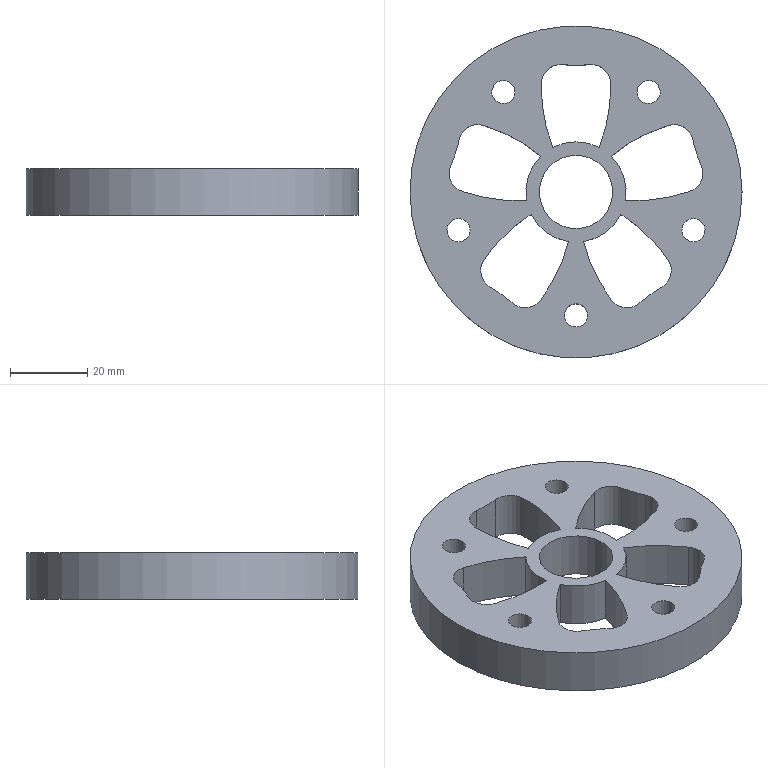Part | NX | features DATUM_CSYS 4, EXTRUDE 4, SKETCH 3 | 1 solid | 39 faces | box 86 x 86 x 12 mm | volume 44699 mm3 | cylinder 37 | plane 2 | commonest cylinder face diameters 86 x11 10 x10 6 x5 26 x5 70 x5 19 x1
STEP:
#1=CARTESIAN_POINT('',(43.,0.,-12.));
#2=VERTEX_POINT('',#1);
#3=CARTESIAN_POINT('',(0.,0.,-12.));
#4=DIRECTION('',(0.,0.,1.));
#5=DIRECTION('',(1.,0.,0.));
#6=AXIS2_PLACEMENT_3D('',#3,#4,#5);
#7=CIRCLE('',#6,43.);
#8=EDGE_CURVE('',#2,#2,#7,.T.);
#9=ORIENTED_EDGE('',*,*,#8,.T.);
#10=EDGE_LOOP('',(#9));
#11=FACE_BOUND('',#10,.T.);
#12=CARTESIAN_POINT('',(43.,0.,0.));
#13=VERTEX_POINT('',#12);
#14=CARTESIAN_POINT('',(0.,0.,0.));
#15=DIRECTION('',(0.,0.,1.));
#16=DIRECTION('',(1.,0.,0.));
#17=AXIS2_PLACEMENT_3D('',#14,#15,#16);
#18=CIRCLE('',#17,43.);
#19=EDGE_CURVE('',#13,#13,#18,.T.);
#20=ORIENTED_EDGE('',*,*,#19,.F.);
#21=EDGE_LOOP('',(#20));
#22=FACE_BOUND('',#21,.T.);
#23=CARTESIAN_POINT('',(0.,0.,-12.));
#24=DIRECTION('',(0.,0.,1.));
#25=DIRECTION('',(1.,0.,0.));
#26=AXIS2_PLACEMENT_3D('',#23,#24,#25);
#27=CYLINDRICAL_SURFACE('',#26,43.);
#28=ADVANCED_FACE('',(#11,#22),#27,.T.);
#29=CARTESIAN_POINT('',(9.5,0.,-12.));
#30=VERTEX_POINT('',#29);
#31=CARTESIAN_POINT('',(0.,0.,-12.));
#32=DIRECTION('',(0.,0.,1.));
#33=DIRECTION('',(1.,0.,0.));
#34=AXIS2_PLACEMENT_3D('',#31,#32,#33);
#35=CIRCLE('',#34,9.5);
#36=EDGE_CURVE('',#30,#30,#35,.T.);
#37=ORIENTED_EDGE('',*,*,#36,.F.);
#38=EDGE_LOOP('',(#37));
#39=FACE_BOUND('',#38,.T.);
#40=CARTESIAN_POINT('',(9.5,0.,0.));
#41=VERTEX_POINT('',#40);
#42=CARTESIAN_POINT('',(0.,0.,0.));
#43=DIRECTION('',(0.,0.,1.));
#44=DIRECTION('',(1.,0.,0.));
#45=AXIS2_PLACEMENT_3D('',#42,#43,#44);
#46=CIRCLE('',#45,9.5);
#47=EDGE_CURVE('',#41,#41,#46,.T.);
#48=ORIENTED_EDGE('',*,*,#47,.T.);
#49=EDGE_LOOP('',(#48));
#50=FACE_BOUND('',#49,.T.);
#51=CARTESIAN_POINT('',(0.,0.,-12.));
#52=DIRECTION('',(0.,0.,1.));
#53=DIRECTION('',(1.,0.,0.));
#54=AXIS2_PLACEMENT_3D('',#51,#52,#53);
#55=CYLINDRICAL_SURFACE('',#54,9.5);
#56=ADVANCED_FACE('',(#39,#50),#55,.F.);
#57=CARTESIAN_POINT('',(31.361,-7.035,-12.));
#58=VERTEX_POINT('',#57);
#59=CARTESIAN_POINT('',(30.434,-9.889,-12.));
#60=DIRECTION('',(0.,0.,1.));
#61=DIRECTION('',(0.309,0.9511,0.));
#62=AXIS2_PLACEMENT_3D('',#59,#60,#61);
#63=CIRCLE('',#62,3.);
#64=EDGE_CURVE('',#58,#58,#63,.T.);
#65=ORIENTED_EDGE('',*,*,#64,.T.);
#66=EDGE_LOOP('',(#65));
#67=FACE_BOUND('',#66,.T.);
#68=CARTESIAN_POINT('',(16.382,27.652,-12.));
#69=VERTEX_POINT('',#68);
#70=CARTESIAN_POINT('',(18.809,25.889,-12.));
#71=DIRECTION('',(0.,0.,1.));
#72=DIRECTION('',(-0.809,0.5878,0.));
#73=AXIS2_PLACEMENT_3D('',#70,#71,#72);
#74=CIRCLE('',#73,3.);
#75=EDGE_CURVE('',#69,#69,#74,.T.);
#76=ORIENTED_EDGE('',*,*,#75,.T.);
#77=EDGE_LOOP('',(#76));
#78=FACE_BOUND('',#77,.T.);
#79=CARTESIAN_POINT('',(3.,-32.,-12.));
#80=VERTEX_POINT('',#79);
#81=CARTESIAN_POINT('',(0.,-32.,-12.));
#82=DIRECTION('',(0.,0.,1.));
#83=DIRECTION('',(1.,0.,0.));
#84=AXIS2_PLACEMENT_3D('',#81,#82,#83);
#85=CIRCLE('',#84,3.);
#86=EDGE_CURVE('',#80,#80,#85,.T.);
#87=ORIENTED_EDGE('',*,*,#86,.T.);
#88=EDGE_LOOP('',(#87));
#89=FACE_BOUND('',#88,.T.);
#90=CARTESIAN_POINT('',(-21.236,24.125,-12.));
#91=VERTEX_POINT('',#90);
#92=CARTESIAN_POINT('',(-18.809,25.889,-12.));
#93=DIRECTION('',(0.,0.,1.));
#94=DIRECTION('',(-0.809,-0.5878,0.));
#95=AXIS2_PLACEMENT_3D('',#92,#93,#94);
#96=CIRCLE('',#95,3.);
#97=EDGE_CURVE('',#91,#91,#96,.T.);
#98=ORIENTED_EDGE('',*,*,#97,.T.);
#99=EDGE_LOOP('',(#98));
#100=FACE_BOUND('',#99,.T.);
#101=CARTESIAN_POINT('',(-29.507,-12.742,-12.));
#102=VERTEX_POINT('',#101);
#103=CARTESIAN_POINT('',(-30.434,-9.889,-12.));
#104=DIRECTION('',(0.,0.,1.));
#105=DIRECTION('',(0.309,-0.9511,0.));
#106=AXIS2_PLACEMENT_3D('',#103,#104,#105);
#107=CIRCLE('',#106,3.);
#108=EDGE_CURVE('',#102,#102,#107,.T.);
#109=ORIENTED_EDGE('',*,*,#108,.T.);
#110=EDGE_LOOP('',(#109));
#111=FACE_BOUND('',#110,.T.);
#112=CARTESIAN_POINT('',(-23.933,17.239,-12.));
#113=VERTEX_POINT('',#112);
#114=CARTESIAN_POINT('',(-30.279,13.519,-12.));
#115=VERTEX_POINT('',#114);
#116=CARTESIAN_POINT('',(-25.394,12.457,-12.));
#117=DIRECTION('',(0.,0.,1.));
#118=DIRECTION('',(1.,0.,0.));
#119=AXIS2_PLACEMENT_3D('',#116,#117,#118);
#120=CIRCLE('',#119,5.);
#121=EDGE_CURVE('',#113,#115,#120,.T.);
#122=ORIENTED_EDGE('',*,*,#121,.T.);
#123=CARTESIAN_POINT('',(-32.443,6.861,-12.));
#124=VERTEX_POINT('',#123);
#125=CARTESIAN_POINT('',(-64.481,20.951,-12.));
#126=DIRECTION('',(0.,0.,1.));
#127=DIRECTION('',(1.,0.,0.));
#128=AXIS2_PLACEMENT_3D('',#125,#126,#127);
#129=CIRCLE('',#128,35.);
#130=EDGE_CURVE('',#115,#124,#129,.F.);
#131=ORIENTED_EDGE('',*,*,#130,.T.);
#132=CARTESIAN_POINT('',(-29.495,0.1211,-12.));
#133=VERTEX_POINT('',#132);
#134=CARTESIAN_POINT('',(-27.866,4.848,-12.));
#135=DIRECTION('',(0.,0.,1.));
#136=DIRECTION('',(1.,0.,0.));
#137=AXIS2_PLACEMENT_3D('',#134,#135,#136);
#138=CIRCLE('',#137,5.);
#139=EDGE_CURVE('',#124,#133,#138,.T.);
#140=ORIENTED_EDGE('',*,*,#139,.T.);
#141=CARTESIAN_POINT('',(-12.822,-2.143,-12.));
#142=VERTEX_POINT('',#141);
#143=CARTESIAN_POINT('',(-15.485,40.775,-12.));
#144=DIRECTION('',(0.,0.,1.));
#145=DIRECTION('',(1.,0.,0.));
#146=AXIS2_PLACEMENT_3D('',#143,#144,#145);
#147=CIRCLE('',#146,43.);
#148=EDGE_CURVE('',#133,#142,#147,.T.);
#149=ORIENTED_EDGE('',*,*,#148,.T.);
#150=CARTESIAN_POINT('',(-9.114,9.27,-12.));
#151=VERTEX_POINT('',#150);
#152=CARTESIAN_POINT('',(0.,0.,-12.));
#153=DIRECTION('',(0.,0.,1.));
#154=DIRECTION('',(1.,0.,0.));
#155=AXIS2_PLACEMENT_3D('',#152,#153,#154);
#156=CIRCLE('',#155,13.);
#157=EDGE_CURVE('',#142,#151,#156,.F.);
#158=ORIENTED_EDGE('',*,*,#157,.T.);
#159=CARTESIAN_POINT('',(-36.495,-23.886,-12.));
#160=DIRECTION('',(0.,0.,1.));
#161=DIRECTION('',(1.,0.,0.));
#162=AXIS2_PLACEMENT_3D('',#159,#160,#161);
#163=CIRCLE('',#162,43.);
#164=EDGE_CURVE('',#151,#113,#163,.T.);
#165=ORIENTED_EDGE('',*,*,#164,.T.);
#166=EDGE_LOOP('',(#122,#131,#140,#149,#158,#165));
#167=FACE_BOUND('',#166,.T.);
#168=CARTESIAN_POINT('',(-11.633,-5.803,-12.));
#169=VERTEX_POINT('',#168);
#170=CARTESIAN_POINT('',(-23.791,-17.434,-12.));
#171=VERTEX_POINT('',#170);
#172=CARTESIAN_POINT('',(11.439,-42.09,-12.));
#173=DIRECTION('',(0.,0.,1.));
#174=DIRECTION('',(1.,0.,0.));
#175=AXIS2_PLACEMENT_3D('',#172,#173,#174);
#176=CIRCLE('',#175,43.);
#177=EDGE_CURVE('',#169,#171,#176,.T.);
#178=ORIENTED_EDGE('',*,*,#177,.T.);
#179=CARTESIAN_POINT('',(-22.214,-24.62,-12.));
#180=VERTEX_POINT('',#179);
#181=CARTESIAN_POINT('',(-19.694,-20.301,-12.));
#182=DIRECTION('',(0.,0.,1.));
#183=DIRECTION('',(1.,0.,0.));
#184=AXIS2_PLACEMENT_3D('',#181,#182,#183);
#185=CIRCLE('',#184,5.);
#186=EDGE_CURVE('',#171,#180,#185,.T.);
#187=ORIENTED_EDGE('',*,*,#186,.T.);
#188=CARTESIAN_POINT('',(-16.551,-28.735,-12.));
#189=VERTEX_POINT('',#188);
#190=CARTESIAN_POINT('',(-39.852,-54.851,-12.));
#191=DIRECTION('',(0.,0.,1.));
#192=DIRECTION('',(1.,0.,0.));
#193=AXIS2_PLACEMENT_3D('',#190,#191,#192);
#194=CIRCLE('',#193,35.);
#195=EDGE_CURVE('',#180,#189,#194,.F.);
#196=ORIENTED_EDGE('',*,*,#195,.T.);
#197=CARTESIAN_POINT('',(-9.229,-28.014,-12.));
#198=VERTEX_POINT('',#197);
#199=CARTESIAN_POINT('',(-13.222,-25.004,-12.));
#200=DIRECTION('',(0.,0.,1.));
#201=DIRECTION('',(1.,0.,0.));
#202=AXIS2_PLACEMENT_3D('',#199,#200,#201);
#203=CIRCLE('',#202,5.);
#204=EDGE_CURVE('',#189,#198,#203,.T.);
#205=ORIENTED_EDGE('',*,*,#204,.T.);
#206=CARTESIAN_POINT('',(-1.925,-12.857,-12.));
#207=VERTEX_POINT('',#206);
#208=CARTESIAN_POINT('',(-43.564,-2.127,-12.));
#209=DIRECTION('',(0.,0.,1.));
#210=DIRECTION('',(1.,0.,0.));
#211=AXIS2_PLACEMENT_3D('',#208,#209,#210);
#212=CIRCLE('',#211,43.);
#213=EDGE_CURVE('',#198,#207,#212,.T.);
#214=ORIENTED_EDGE('',*,*,#213,.T.);
#215=CARTESIAN_POINT('',(0.,0.,-12.));
#216=DIRECTION('',(0.,0.,1.));
#217=DIRECTION('',(1.,0.,0.));
#218=AXIS2_PLACEMENT_3D('',#215,#216,#217);
#219=CIRCLE('',#218,13.);
#220=EDGE_CURVE('',#207,#169,#219,.F.);
#221=ORIENTED_EDGE('',*,*,#220,.T.);
#222=EDGE_LOOP('',(#178,#187,#196,#205,#214,#221));
#223=FACE_BOUND('',#222,.T.);
#224=CARTESIAN_POINT('',(-8.999,28.089,-12.));
#225=VERTEX_POINT('',#224);
#226=CARTESIAN_POINT('',(-6.,11.533,-12.));
#227=VERTEX_POINT('',#226);
#228=CARTESIAN_POINT('',(33.994,27.327,-12.));
#229=DIRECTION('',(0.,0.,1.));
#230=DIRECTION('',(1.,0.,0.));
#231=AXIS2_PLACEMENT_3D('',#228,#229,#230);
#232=CIRCLE('',#231,43.);
#233=EDGE_CURVE('',#225,#227,#232,.T.);
#234=ORIENTED_EDGE('',*,*,#233,.T.);
#235=CARTESIAN_POINT('',(6.,11.533,-12.));
#236=VERTEX_POINT('',#235);
#237=CARTESIAN_POINT('',(0.,0.,-12.));
#238=DIRECTION('',(0.,0.,1.));
#239=DIRECTION('',(1.,0.,0.));
#240=AXIS2_PLACEMENT_3D('',#237,#238,#239);
#241=CIRCLE('',#240,13.);
#242=EDGE_CURVE('',#227,#236,#241,.F.);
#243=ORIENTED_EDGE('',*,*,#242,.T.);
#244=CARTESIAN_POINT('',(8.999,28.089,-12.));
#245=VERTEX_POINT('',#244);
#246=CARTESIAN_POINT('',(-33.994,27.327,-12.));
#247=DIRECTION('',(0.,0.,1.));
#248=DIRECTION('',(1.,0.,0.));
#249=AXIS2_PLACEMENT_3D('',#246,#247,#248);
#250=CIRCLE('',#249,43.);
#251=EDGE_CURVE('',#236,#245,#250,.T.);
#252=ORIENTED_EDGE('',*,*,#251,.T.);
#253=CARTESIAN_POINT('',(3.5,32.975,-12.));
#254=VERTEX_POINT('',#253);
#255=CARTESIAN_POINT('',(4.,28.,-12.));
#256=DIRECTION('',(0.,0.,1.));
#257=DIRECTION('',(1.,0.,0.));
#258=AXIS2_PLACEMENT_3D('',#255,#256,#257);
#259=CIRCLE('',#258,5.);
#260=EDGE_CURVE('',#245,#254,#259,.T.);
#261=ORIENTED_EDGE('',*,*,#260,.T.);
#262=CARTESIAN_POINT('',(-3.5,32.975,-12.));
#263=VERTEX_POINT('',#262);
#264=CARTESIAN_POINT('',(0.,67.799,-12.));
#265=DIRECTION('',(0.,0.,1.));
#266=DIRECTION('',(1.,0.,0.));
#267=AXIS2_PLACEMENT_3D('',#264,#265,#266);
#268=CIRCLE('',#267,35.);
#269=EDGE_CURVE('',#254,#263,#268,.F.);
#270=ORIENTED_EDGE('',*,*,#269,.T.);
#271=CARTESIAN_POINT('',(-4.,28.,-12.));
#272=DIRECTION('',(0.,0.,1.));
#273=DIRECTION('',(1.,0.,0.));
#274=AXIS2_PLACEMENT_3D('',#271,#272,#273);
#275=CIRCLE('',#274,5.);
#276=EDGE_CURVE('',#263,#225,#275,.T.);
#277=ORIENTED_EDGE('',*,*,#276,.T.);
#278=EDGE_LOOP('',(#234,#243,#252,#261,#270,#277));
#279=FACE_BOUND('',#278,.T.);
#280=CARTESIAN_POINT('',(11.633,-5.803,-12.));
#281=VERTEX_POINT('',#280);
#282=CARTESIAN_POINT('',(1.925,-12.857,-12.));
#283=VERTEX_POINT('',#282);
#284=CARTESIAN_POINT('',(0.,0.,-12.));
#285=DIRECTION('',(0.,0.,1.));
#286=DIRECTION('',(1.,0.,0.));
#287=AXIS2_PLACEMENT_3D('',#284,#285,#286);
#288=CIRCLE('',#287,13.);
#289=EDGE_CURVE('',#281,#283,#288,.F.);
#290=ORIENTED_EDGE('',*,*,#289,.T.);
#291=CARTESIAN_POINT('',(9.229,-28.014,-12.));
#292=VERTEX_POINT('',#291);
#293=CARTESIAN_POINT('',(43.564,-2.127,-12.));
#294=DIRECTION('',(0.,0.,1.));
#295=DIRECTION('',(1.,0.,0.));
#296=AXIS2_PLACEMENT_3D('',#293,#294,#295);
#297=CIRCLE('',#296,43.);
#298=EDGE_CURVE('',#283,#292,#297,.T.);
#299=ORIENTED_EDGE('',*,*,#298,.T.);
#300=CARTESIAN_POINT('',(16.551,-28.735,-12.));
#301=VERTEX_POINT('',#300);
#302=CARTESIAN_POINT('',(13.222,-25.004,-12.));
#303=DIRECTION('',(0.,0.,1.));
#304=DIRECTION('',(1.,0.,0.));
#305=AXIS2_PLACEMENT_3D('',#302,#303,#304);
#306=CIRCLE('',#305,5.);
#307=EDGE_CURVE('',#292,#301,#306,.T.);
#308=ORIENTED_EDGE('',*,*,#307,.T.);
#309=CARTESIAN_POINT('',(22.214,-24.62,-12.));
#310=VERTEX_POINT('',#309);
#311=CARTESIAN_POINT('',(39.852,-54.851,-12.));
#312=DIRECTION('',(0.,0.,1.));
#313=DIRECTION('',(1.,0.,0.));
#314=AXIS2_PLACEMENT_3D('',#311,#312,#313);
#315=CIRCLE('',#314,35.);
#316=EDGE_CURVE('',#301,#310,#315,.F.);
#317=ORIENTED_EDGE('',*,*,#316,.T.);
#318=CARTESIAN_POINT('',(23.791,-17.434,-12.));
#319=VERTEX_POINT('',#318);
#320=CARTESIAN_POINT('',(19.694,-20.301,-12.));
#321=DIRECTION('',(0.,0.,1.));
#322=DIRECTION('',(1.,0.,0.));
#323=AXIS2_PLACEMENT_3D('',#320,#321,#322);
#324=CIRCLE('',#323,5.);
#325=EDGE_CURVE('',#310,#319,#324,.T.);
#326=ORIENTED_EDGE('',*,*,#325,.T.);
#327=CARTESIAN_POINT('',(-11.439,-42.09,-12.));
#328=DIRECTION('',(0.,0.,1.));
#329=DIRECTION('',(1.,0.,0.));
#330=AXIS2_PLACEMENT_3D('',#327,#328,#329);
#331=CIRCLE('',#330,43.);
#332=EDGE_CURVE('',#319,#281,#331,.T.);
#333=ORIENTED_EDGE('',*,*,#332,.T.);
#334=EDGE_LOOP('',(#290,#299,#308,#317,#326,#333));
#335=FACE_BOUND('',#334,.T.);
#336=CARTESIAN_POINT('',(23.933,17.239,-12.));
#337=VERTEX_POINT('',#336);
#338=CARTESIAN_POINT('',(9.114,9.27,-12.));
#339=VERTEX_POINT('',#338);
#340=CARTESIAN_POINT('',(36.495,-23.886,-12.));
#341=DIRECTION('',(0.,0.,1.));
#342=DIRECTION('',(1.,0.,0.));
#343=AXIS2_PLACEMENT_3D('',#340,#341,#342);
#344=CIRCLE('',#343,43.);
#345=EDGE_CURVE('',#337,#339,#344,.T.);
#346=ORIENTED_EDGE('',*,*,#345,.T.);
#347=CARTESIAN_POINT('',(12.822,-2.143,-12.));
#348=VERTEX_POINT('',#347);
#349=CARTESIAN_POINT('',(0.,0.,-12.));
#350=DIRECTION('',(0.,0.,1.));
#351=DIRECTION('',(1.,0.,0.));
#352=AXIS2_PLACEMENT_3D('',#349,#350,#351);
#353=CIRCLE('',#352,13.);
#354=EDGE_CURVE('',#339,#348,#353,.F.);
#355=ORIENTED_EDGE('',*,*,#354,.T.);
#356=CARTESIAN_POINT('',(29.495,0.1211,-12.));
#357=VERTEX_POINT('',#356);
#358=CARTESIAN_POINT('',(15.485,40.775,-12.));
#359=DIRECTION('',(0.,0.,1.));
#360=DIRECTION('',(1.,0.,0.));
#361=AXIS2_PLACEMENT_3D('',#358,#359,#360);
#362=CIRCLE('',#361,43.);
#363=EDGE_CURVE('',#348,#357,#362,.T.);
#364=ORIENTED_EDGE('',*,*,#363,.T.);
#365=CARTESIAN_POINT('',(32.443,6.861,-12.));
#366=VERTEX_POINT('',#365);
#367=CARTESIAN_POINT('',(27.866,4.848,-12.));
#368=DIRECTION('',(0.,0.,1.));
#369=DIRECTION('',(1.,0.,0.));
#370=AXIS2_PLACEMENT_3D('',#367,#368,#369);
#371=CIRCLE('',#370,5.);
#372=EDGE_CURVE('',#357,#366,#371,.T.);
#373=ORIENTED_EDGE('',*,*,#372,.T.);
#374=CARTESIAN_POINT('',(30.279,13.519,-12.));
#375=VERTEX_POINT('',#374);
#376=CARTESIAN_POINT('',(64.481,20.951,-12.));
#377=DIRECTION('',(0.,0.,1.));
#378=DIRECTION('',(1.,0.,0.));
#379=AXIS2_PLACEMENT_3D('',#376,#377,#378);
#380=CIRCLE('',#379,35.);
#381=EDGE_CURVE('',#366,#375,#380,.F.);
#382=ORIENTED_EDGE('',*,*,#381,.T.);
#383=CARTESIAN_POINT('',(25.394,12.457,-12.));
#384=DIRECTION('',(0.,0.,1.));
#385=DIRECTION('',(1.,0.,0.));
#386=AXIS2_PLACEMENT_3D('',#383,#384,#385);
#387=CIRCLE('',#386,5.);
#388=EDGE_CURVE('',#375,#337,#387,.T.);
#389=ORIENTED_EDGE('',*,*,#388,.T.);
#390=EDGE_LOOP('',(#346,#355,#364,#373,#382,#389));
#391=FACE_BOUND('',#390,.T.);
#392=ORIENTED_EDGE('',*,*,#8,.F.);
#393=EDGE_LOOP('',(#392));
#394=FACE_BOUND('',#393,.T.);
#395=ORIENTED_EDGE('',*,*,#36,.T.);
#396=EDGE_LOOP('',(#395));
#397=FACE_BOUND('',#396,.T.);
#398=CARTESIAN_POINT('',(0.,0.,-12.));
#399=DIRECTION('',(0.,0.,1.));
#400=DIRECTION('',(1.,0.,0.));
#401=AXIS2_PLACEMENT_3D('',#398,#399,#400);
#402=PLANE('',#401);
#403=ADVANCED_FACE('',(#67,#78,#89,#100,#111,#167,#223,#279,#335,#391,#394,#397),#402,.F.);
#404=CARTESIAN_POINT('',(9.114,9.27,0.));
#405=VERTEX_POINT('',#404);
#406=CARTESIAN_POINT('',(12.822,-2.143,0.));
#407=VERTEX_POINT('',#406);
#408=CARTESIAN_POINT('',(0.,0.,0.));
#409=DIRECTION('',(0.,0.,-1.));
#410=DIRECTION('',(0.309,-0.9511,0.));
#411=AXIS2_PLACEMENT_3D('',#408,#409,#410);
#412=CIRCLE('',#411,13.);
#413=EDGE_CURVE('',#405,#407,#412,.T.);
#414=ORIENTED_EDGE('',*,*,#413,.F.);
#415=CARTESIAN_POINT('',(23.933,17.239,0.));
#416=VERTEX_POINT('',#415);
#417=CARTESIAN_POINT('',(36.495,-23.886,0.));
#418=DIRECTION('',(0.,0.,1.));
#419=DIRECTION('',(0.309,-0.9511,0.));
#420=AXIS2_PLACEMENT_3D('',#417,#418,#419);
#421=CIRCLE('',#420,43.);
#422=EDGE_CURVE('',#416,#405,#421,.T.);
#423=ORIENTED_EDGE('',*,*,#422,.F.);
#424=CARTESIAN_POINT('',(30.279,13.519,0.));
#425=VERTEX_POINT('',#424);
#426=CARTESIAN_POINT('',(25.394,12.457,0.));
#427=DIRECTION('',(0.,0.,1.));
#428=DIRECTION('',(0.309,-0.9511,0.));
#429=AXIS2_PLACEMENT_3D('',#426,#427,#428);
#430=CIRCLE('',#429,5.);
#431=EDGE_CURVE('',#425,#416,#430,.T.);
#432=ORIENTED_EDGE('',*,*,#431,.F.);
#433=CARTESIAN_POINT('',(32.443,6.861,0.));
#434=VERTEX_POINT('',#433);
#435=CARTESIAN_POINT('',(64.481,20.951,0.));
#436=DIRECTION('',(0.,0.,-1.));
#437=DIRECTION('',(0.309,-0.9511,0.));
#438=AXIS2_PLACEMENT_3D('',#435,#436,#437);
#439=CIRCLE('',#438,35.);
#440=EDGE_CURVE('',#434,#425,#439,.T.);
#441=ORIENTED_EDGE('',*,*,#440,.F.);
#442=CARTESIAN_POINT('',(29.495,0.1211,0.));
#443=VERTEX_POINT('',#442);
#444=CARTESIAN_POINT('',(27.866,4.848,0.));
#445=DIRECTION('',(0.,0.,1.));
#446=DIRECTION('',(-0.309,0.9511,0.));
#447=AXIS2_PLACEMENT_3D('',#444,#445,#446);
#448=CIRCLE('',#447,5.);
#449=EDGE_CURVE('',#443,#434,#448,.T.);
#450=ORIENTED_EDGE('',*,*,#449,.F.);
#451=CARTESIAN_POINT('',(15.485,40.775,0.));
#452=DIRECTION('',(0.,0.,1.));
#453=DIRECTION('',(-0.309,0.9511,0.));
#454=AXIS2_PLACEMENT_3D('',#451,#452,#453);
#455=CIRCLE('',#454,43.);
#456=EDGE_CURVE('',#407,#443,#455,.T.);
#457=ORIENTED_EDGE('',*,*,#456,.F.);
#458=EDGE_LOOP('',(#414,#423,#432,#441,#450,#457));
#459=FACE_BOUND('',#458,.T.);
#460=CARTESIAN_POINT('',(-3.5,32.975,0.));
#461=VERTEX_POINT('',#460);
#462=CARTESIAN_POINT('',(-8.999,28.089,0.));
#463=VERTEX_POINT('',#462);
#464=CARTESIAN_POINT('',(-4.,28.,0.));
#465=DIRECTION('',(0.,0.,1.));
#466=DIRECTION('',(1.,0.,0.));
#467=AXIS2_PLACEMENT_3D('',#464,#465,#466);
#468=CIRCLE('',#467,5.);
#469=EDGE_CURVE('',#461,#463,#468,.T.);
#470=ORIENTED_EDGE('',*,*,#469,.F.);
#471=CARTESIAN_POINT('',(3.5,32.975,0.));
#472=VERTEX_POINT('',#471);
#473=CARTESIAN_POINT('',(0.,67.799,0.));
#474=DIRECTION('',(0.,0.,-1.));
#475=DIRECTION('',(1.,0.,0.));
#476=AXIS2_PLACEMENT_3D('',#473,#474,#475);
#477=CIRCLE('',#476,35.);
#478=EDGE_CURVE('',#472,#461,#477,.T.);
#479=ORIENTED_EDGE('',*,*,#478,.F.);
#480=CARTESIAN_POINT('',(8.999,28.089,0.));
#481=VERTEX_POINT('',#480);
#482=CARTESIAN_POINT('',(4.,28.,0.));
#483=DIRECTION('',(0.,0.,1.));
#484=DIRECTION('',(-1.,0.,0.));
#485=AXIS2_PLACEMENT_3D('',#482,#483,#484);
#486=CIRCLE('',#485,5.);
#487=EDGE_CURVE('',#481,#472,#486,.T.);
#488=ORIENTED_EDGE('',*,*,#487,.F.);
#489=CARTESIAN_POINT('',(6.,11.533,0.));
#490=VERTEX_POINT('',#489);
#491=CARTESIAN_POINT('',(-33.994,27.327,0.));
#492=DIRECTION('',(0.,0.,1.));
#493=DIRECTION('',(-1.,0.,0.));
#494=AXIS2_PLACEMENT_3D('',#491,#492,#493);
#495=CIRCLE('',#494,43.);
#496=EDGE_CURVE('',#490,#481,#495,.T.);
#497=ORIENTED_EDGE('',*,*,#496,.F.);
#498=CARTESIAN_POINT('',(-6.,11.533,0.));
#499=VERTEX_POINT('',#498);
#500=CARTESIAN_POINT('',(0.,0.,0.));
#501=DIRECTION('',(0.,0.,-1.));
#502=DIRECTION('',(1.,0.,0.));
#503=AXIS2_PLACEMENT_3D('',#500,#501,#502);
#504=CIRCLE('',#503,13.);
#505=EDGE_CURVE('',#499,#490,#504,.T.);
#506=ORIENTED_EDGE('',*,*,#505,.F.);
#507=CARTESIAN_POINT('',(33.994,27.327,0.));
#508=DIRECTION('',(0.,0.,1.));
#509=DIRECTION('',(1.,0.,0.));
#510=AXIS2_PLACEMENT_3D('',#507,#508,#509);
#511=CIRCLE('',#510,43.);
#512=EDGE_CURVE('',#463,#499,#511,.T.);
#513=ORIENTED_EDGE('',*,*,#512,.F.);
#514=EDGE_LOOP('',(#470,#479,#488,#497,#506,#513));
#515=FACE_BOUND('',#514,.T.);
#516=CARTESIAN_POINT('',(31.361,-7.035,0.));
#517=VERTEX_POINT('',#516);
#518=CARTESIAN_POINT('',(30.434,-9.889,0.));
#519=DIRECTION('',(0.,0.,1.));
#520=DIRECTION('',(0.309,0.9511,0.));
#521=AXIS2_PLACEMENT_3D('',#518,#519,#520);
#522=CIRCLE('',#521,3.);
#523=EDGE_CURVE('',#517,#517,#522,.T.);
#524=ORIENTED_EDGE('',*,*,#523,.F.);
#525=EDGE_LOOP('',(#524));
#526=FACE_BOUND('',#525,.T.);
#527=CARTESIAN_POINT('',(16.382,27.652,0.));
#528=VERTEX_POINT('',#527);
#529=CARTESIAN_POINT('',(18.809,25.889,0.));
#530=DIRECTION('',(0.,0.,1.));
#531=DIRECTION('',(-0.809,0.5878,0.));
#532=AXIS2_PLACEMENT_3D('',#529,#530,#531);
#533=CIRCLE('',#532,3.);
#534=EDGE_CURVE('',#528,#528,#533,.T.);
#535=ORIENTED_EDGE('',*,*,#534,.F.);
#536=EDGE_LOOP('',(#535));
#537=FACE_BOUND('',#536,.T.);
#538=CARTESIAN_POINT('',(3.,-32.,0.));
#539=VERTEX_POINT('',#538);
#540=CARTESIAN_POINT('',(0.,-32.,0.));
#541=DIRECTION('',(0.,0.,1.));
#542=DIRECTION('',(1.,0.,0.));
#543=AXIS2_PLACEMENT_3D('',#540,#541,#542);
#544=CIRCLE('',#543,3.);
#545=EDGE_CURVE('',#539,#539,#544,.T.);
#546=ORIENTED_EDGE('',*,*,#545,.F.);
#547=EDGE_LOOP('',(#546));
#548=FACE_BOUND('',#547,.T.);
#549=CARTESIAN_POINT('',(-21.236,24.125,0.));
#550=VERTEX_POINT('',#549);
#551=CARTESIAN_POINT('',(-18.809,25.889,0.));
#552=DIRECTION('',(0.,0.,1.));
#553=DIRECTION('',(-0.809,-0.5878,0.));
#554=AXIS2_PLACEMENT_3D('',#551,#552,#553);
#555=CIRCLE('',#554,3.);
#556=EDGE_CURVE('',#550,#550,#555,.T.);
#557=ORIENTED_EDGE('',*,*,#556,.F.);
#558=EDGE_LOOP('',(#557));
#559=FACE_BOUND('',#558,.T.);
#560=CARTESIAN_POINT('',(-29.507,-12.742,0.));
#561=VERTEX_POINT('',#560);
#562=CARTESIAN_POINT('',(-30.434,-9.889,0.));
#563=DIRECTION('',(0.,0.,1.));
#564=DIRECTION('',(0.309,-0.9511,0.));
#565=AXIS2_PLACEMENT_3D('',#562,#563,#564);
#566=CIRCLE('',#565,3.);
#567=EDGE_CURVE('',#561,#561,#566,.T.);
#568=ORIENTED_EDGE('',*,*,#567,.F.);
#569=EDGE_LOOP('',(#568));
#570=FACE_BOUND('',#569,.T.);
#571=CARTESIAN_POINT('',(-30.279,13.519,0.));
#572=VERTEX_POINT('',#571);
#573=CARTESIAN_POINT('',(-32.443,6.861,0.));
#574=VERTEX_POINT('',#573);
#575=CARTESIAN_POINT('',(-64.481,20.951,0.));
#576=DIRECTION('',(0.,0.,-1.));
#577=DIRECTION('',(0.309,0.9511,0.));
#578=AXIS2_PLACEMENT_3D('',#575,#576,#577);
#579=CIRCLE('',#578,35.);
#580=EDGE_CURVE('',#572,#574,#579,.T.);
#581=ORIENTED_EDGE('',*,*,#580,.F.);
#582=CARTESIAN_POINT('',(-23.933,17.239,0.));
#583=VERTEX_POINT('',#582);
#584=CARTESIAN_POINT('',(-25.394,12.457,0.));
#585=DIRECTION('',(0.,0.,1.));
#586=DIRECTION('',(-0.309,-0.9511,0.));
#587=AXIS2_PLACEMENT_3D('',#584,#585,#586);
#588=CIRCLE('',#587,5.);
#589=EDGE_CURVE('',#583,#572,#588,.T.);
#590=ORIENTED_EDGE('',*,*,#589,.F.);
#591=CARTESIAN_POINT('',(-9.114,9.27,0.));
#592=VERTEX_POINT('',#591);
#593=CARTESIAN_POINT('',(-36.495,-23.886,0.));
#594=DIRECTION('',(0.,0.,1.));
#595=DIRECTION('',(-0.309,-0.9511,0.));
#596=AXIS2_PLACEMENT_3D('',#593,#594,#595);
#597=CIRCLE('',#596,43.);
#598=EDGE_CURVE('',#592,#583,#597,.T.);
#599=ORIENTED_EDGE('',*,*,#598,.F.);
#600=CARTESIAN_POINT('',(-12.822,-2.143,0.));
#601=VERTEX_POINT('',#600);
#602=CARTESIAN_POINT('',(0.,0.,0.));
#603=DIRECTION('',(0.,0.,-1.));
#604=DIRECTION('',(0.309,0.9511,0.));
#605=AXIS2_PLACEMENT_3D('',#602,#603,#604);
#606=CIRCLE('',#605,13.);
#607=EDGE_CURVE('',#601,#592,#606,.T.);
#608=ORIENTED_EDGE('',*,*,#607,.F.);
#609=CARTESIAN_POINT('',(-29.495,0.1211,0.));
#610=VERTEX_POINT('',#609);
#611=CARTESIAN_POINT('',(-15.485,40.775,0.));
#612=DIRECTION('',(0.,0.,1.));
#613=DIRECTION('',(0.309,0.9511,0.));
#614=AXIS2_PLACEMENT_3D('',#611,#612,#613);
#615=CIRCLE('',#614,43.);
#616=EDGE_CURVE('',#610,#601,#615,.T.);
#617=ORIENTED_EDGE('',*,*,#616,.F.);
#618=CARTESIAN_POINT('',(-27.866,4.848,0.));
#619=DIRECTION('',(0.,0.,1.));
#620=DIRECTION('',(0.309,0.9511,0.));
#621=AXIS2_PLACEMENT_3D('',#618,#619,#620);
#622=CIRCLE('',#621,5.);
#623=EDGE_CURVE('',#574,#610,#622,.T.);
#624=ORIENTED_EDGE('',*,*,#623,.F.);
#625=EDGE_LOOP('',(#581,#590,#599,#608,#617,#624));
#626=FACE_BOUND('',#625,.T.);
#627=CARTESIAN_POINT('',(-23.791,-17.434,0.));
#628=VERTEX_POINT('',#627);
#629=CARTESIAN_POINT('',(-22.214,-24.62,0.));
#630=VERTEX_POINT('',#629);
#631=CARTESIAN_POINT('',(-19.694,-20.301,0.));
#632=DIRECTION('',(0.,0.,1.));
#633=DIRECTION('',(0.809,-0.5878,0.));
#634=AXIS2_PLACEMENT_3D('',#631,#632,#633);
#635=CIRCLE('',#634,5.);
#636=EDGE_CURVE('',#628,#630,#635,.T.);
#637=ORIENTED_EDGE('',*,*,#636,.F.);
#638=CARTESIAN_POINT('',(-11.633,-5.803,0.));
#639=VERTEX_POINT('',#638);
#640=CARTESIAN_POINT('',(11.439,-42.09,0.));
#641=DIRECTION('',(0.,0.,1.));
#642=DIRECTION('',(0.809,-0.5878,0.));
#643=AXIS2_PLACEMENT_3D('',#640,#641,#642);
#644=CIRCLE('',#643,43.);
#645=EDGE_CURVE('',#639,#628,#644,.T.);
#646=ORIENTED_EDGE('',*,*,#645,.F.);
#647=CARTESIAN_POINT('',(-1.925,-12.857,0.));
#648=VERTEX_POINT('',#647);
#649=CARTESIAN_POINT('',(0.,0.,0.));
#650=DIRECTION('',(0.,0.,-1.));
#651=DIRECTION('',(-0.809,0.5878,0.));
#652=AXIS2_PLACEMENT_3D('',#649,#650,#651);
#653=CIRCLE('',#652,13.);
#654=EDGE_CURVE('',#648,#639,#653,.T.);
#655=ORIENTED_EDGE('',*,*,#654,.F.);
#656=CARTESIAN_POINT('',(-9.229,-28.014,0.));
#657=VERTEX_POINT('',#656);
#658=CARTESIAN_POINT('',(-43.564,-2.127,0.));
#659=DIRECTION('',(0.,0.,1.));
#660=DIRECTION('',(-0.809,0.5878,0.));
#661=AXIS2_PLACEMENT_3D('',#658,#659,#660);
#662=CIRCLE('',#661,43.);
#663=EDGE_CURVE('',#657,#648,#662,.T.);
#664=ORIENTED_EDGE('',*,*,#663,.F.);
#665=CARTESIAN_POINT('',(-16.551,-28.735,0.));
#666=VERTEX_POINT('',#665);
#667=CARTESIAN_POINT('',(-13.222,-25.004,0.));
#668=DIRECTION('',(0.,0.,1.));
#669=DIRECTION('',(-0.809,0.5878,0.));
#670=AXIS2_PLACEMENT_3D('',#667,#668,#669);
#671=CIRCLE('',#670,5.);
#672=EDGE_CURVE('',#666,#657,#671,.T.);
#673=ORIENTED_EDGE('',*,*,#672,.F.);
#674=CARTESIAN_POINT('',(-39.852,-54.851,0.));
#675=DIRECTION('',(0.,0.,-1.));
#676=DIRECTION('',(-0.809,0.5878,0.));
#677=AXIS2_PLACEMENT_3D('',#674,#675,#676);
#678=CIRCLE('',#677,35.);
#679=EDGE_CURVE('',#630,#666,#678,.T.);
#680=ORIENTED_EDGE('',*,*,#679,.F.);
#681=EDGE_LOOP('',(#637,#646,#655,#664,#673,#680));
#682=FACE_BOUND('',#681,.T.);
#683=CARTESIAN_POINT('',(1.925,-12.857,0.));
#684=VERTEX_POINT('',#683);
#685=CARTESIAN_POINT('',(9.229,-28.014,0.));
#686=VERTEX_POINT('',#685);
#687=CARTESIAN_POINT('',(43.564,-2.127,0.));
#688=DIRECTION('',(0.,0.,1.));
#689=DIRECTION('',(0.809,0.5878,0.));
#690=AXIS2_PLACEMENT_3D('',#687,#688,#689);
#691=CIRCLE('',#690,43.);
#692=EDGE_CURVE('',#684,#686,#691,.T.);
#693=ORIENTED_EDGE('',*,*,#692,.F.);
#694=CARTESIAN_POINT('',(11.633,-5.803,0.));
#695=VERTEX_POINT('',#694);
#696=CARTESIAN_POINT('',(0.,0.,0.));
#697=DIRECTION('',(0.,0.,-1.));
#698=DIRECTION('',(-0.809,-0.5878,0.));
#699=AXIS2_PLACEMENT_3D('',#696,#697,#698);
#700=CIRCLE('',#699,13.);
#701=EDGE_CURVE('',#695,#684,#700,.T.);
#702=ORIENTED_EDGE('',*,*,#701,.F.);
#703=CARTESIAN_POINT('',(23.791,-17.434,0.));
#704=VERTEX_POINT('',#703);
#705=CARTESIAN_POINT('',(-11.439,-42.09,0.));
#706=DIRECTION('',(0.,0.,1.));
#707=DIRECTION('',(-0.809,-0.5878,0.));
#708=AXIS2_PLACEMENT_3D('',#705,#706,#707);
#709=CIRCLE('',#708,43.);
#710=EDGE_CURVE('',#704,#695,#709,.T.);
#711=ORIENTED_EDGE('',*,*,#710,.F.);
#712=CARTESIAN_POINT('',(22.214,-24.62,0.));
#713=VERTEX_POINT('',#712);
#714=CARTESIAN_POINT('',(19.694,-20.301,0.));
#715=DIRECTION('',(0.,0.,1.));
#716=DIRECTION('',(-0.809,-0.5878,0.));
#717=AXIS2_PLACEMENT_3D('',#714,#715,#716);
#718=CIRCLE('',#717,5.);
#719=EDGE_CURVE('',#713,#704,#718,.T.);
#720=ORIENTED_EDGE('',*,*,#719,.F.);
#721=CARTESIAN_POINT('',(16.551,-28.735,0.));
#722=VERTEX_POINT('',#721);
#723=CARTESIAN_POINT('',(39.852,-54.851,0.));
#724=DIRECTION('',(0.,0.,-1.));
#725=DIRECTION('',(-0.809,-0.5878,0.));
#726=AXIS2_PLACEMENT_3D('',#723,#724,#725);
#727=CIRCLE('',#726,35.);
#728=EDGE_CURVE('',#722,#713,#727,.T.);
#729=ORIENTED_EDGE('',*,*,#728,.F.);
#730=CARTESIAN_POINT('',(13.222,-25.004,0.));
#731=DIRECTION('',(0.,0.,1.));
#732=DIRECTION('',(0.809,0.5878,0.));
#733=AXIS2_PLACEMENT_3D('',#730,#731,#732);
#734=CIRCLE('',#733,5.);
#735=EDGE_CURVE('',#686,#722,#734,.T.);
#736=ORIENTED_EDGE('',*,*,#735,.F.);
#737=EDGE_LOOP('',(#693,#702,#711,#720,#729,#736));
#738=FACE_BOUND('',#737,.T.);
#739=ORIENTED_EDGE('',*,*,#19,.T.);
#740=EDGE_LOOP('',(#739));
#741=FACE_BOUND('',#740,.T.);
#742=ORIENTED_EDGE('',*,*,#47,.F.);
#743=EDGE_LOOP('',(#742));
#744=FACE_BOUND('',#743,.T.);
#745=CARTESIAN_POINT('',(0.,0.,0.));
#746=DIRECTION('',(0.,0.,1.));
#747=DIRECTION('',(1.,0.,0.));
#748=AXIS2_PLACEMENT_3D('',#745,#746,#747);
#749=PLANE('',#748);
#750=ADVANCED_FACE('',(#459,#515,#526,#537,#548,#559,#570,#626,#682,#738,#741,#744),#749,.T.);
#751=ORIENTED_EDGE('',*,*,#354,.F.);
#752=CARTESIAN_POINT('',(9.114,9.27,-22.));
#753=DIRECTION('',(0.,0.,1.));
#754=VECTOR('',#753,1000.);
#755=LINE('',#752,#754);
#756=EDGE_CURVE('',#339,#405,#755,.T.);
#757=ORIENTED_EDGE('',*,*,#756,.T.);
#758=ORIENTED_EDGE('',*,*,#413,.T.);
#759=CARTESIAN_POINT('',(12.822,-2.143,-13.2));
#760=DIRECTION('',(0.,0.,1.));
#761=VECTOR('',#760,1000.);
#762=LINE('',#759,#761);
#763=EDGE_CURVE('',#407,#348,#762,.F.);
#764=ORIENTED_EDGE('',*,*,#763,.T.);
#765=EDGE_LOOP('',(#751,#757,#758,#764));
#766=FACE_BOUND('',#765,.T.);
#767=CARTESIAN_POINT('',(0.,0.,-13.2));
#768=DIRECTION('',(0.,0.,1.));
#769=DIRECTION('',(1.,0.,0.));
#770=AXIS2_PLACEMENT_3D('',#767,#768,#769);
#771=CYLINDRICAL_SURFACE('',#770,13.);
#772=ADVANCED_FACE('',(#766),#771,.T.);
#773=ORIENTED_EDGE('',*,*,#763,.F.);
#774=ORIENTED_EDGE('',*,*,#456,.T.);
#775=CARTESIAN_POINT('',(29.495,0.1211,-13.2));
#776=DIRECTION('',(0.,0.,1.));
#777=VECTOR('',#776,1000.);
#778=LINE('',#775,#777);
#779=EDGE_CURVE('',#443,#357,#778,.F.);
#780=ORIENTED_EDGE('',*,*,#779,.T.);
#781=ORIENTED_EDGE('',*,*,#363,.F.);
#782=EDGE_LOOP('',(#773,#774,#780,#781));
#783=FACE_BOUND('',#782,.T.);
#784=CARTESIAN_POINT('',(15.485,40.775,-13.2));
#785=DIRECTION('',(0.,0.,1.));
#786=DIRECTION('',(1.,0.,0.));
#787=AXIS2_PLACEMENT_3D('',#784,#785,#786);
#788=CYLINDRICAL_SURFACE('',#787,43.);
#789=ADVANCED_FACE('',(#783),#788,.F.);
#790=ORIENTED_EDGE('',*,*,#779,.F.);
#791=ORIENTED_EDGE('',*,*,#449,.T.);
#792=CARTESIAN_POINT('',(32.443,6.861,-13.2));
#793=DIRECTION('',(0.,0.,1.));
#794=VECTOR('',#793,1000.);
#795=LINE('',#792,#794);
#796=EDGE_CURVE('',#434,#366,#795,.F.);
#797=ORIENTED_EDGE('',*,*,#796,.T.);
#798=ORIENTED_EDGE('',*,*,#372,.F.);
#799=EDGE_LOOP('',(#790,#791,#797,#798));
#800=FACE_BOUND('',#799,.T.);
#801=CARTESIAN_POINT('',(27.866,4.848,-13.2));
#802=DIRECTION('',(0.,0.,1.));
#803=DIRECTION('',(1.,0.,0.));
#804=AXIS2_PLACEMENT_3D('',#801,#802,#803);
#805=CYLINDRICAL_SURFACE('',#804,5.);
#806=ADVANCED_FACE('',(#800),#805,.F.);
#807=ORIENTED_EDGE('',*,*,#796,.F.);
#808=ORIENTED_EDGE('',*,*,#440,.T.);
#809=CARTESIAN_POINT('',(30.279,13.519,-22.));
#810=DIRECTION('',(0.,0.,1.));
#811=VECTOR('',#810,1000.);
#812=LINE('',#809,#811);
#813=EDGE_CURVE('',#375,#425,#812,.T.);
#814=ORIENTED_EDGE('',*,*,#813,.F.);
#815=ORIENTED_EDGE('',*,*,#381,.F.);
#816=EDGE_LOOP('',(#807,#808,#814,#815));
#817=FACE_BOUND('',#816,.T.);
#818=CARTESIAN_POINT('',(64.481,20.951,-13.2));
#819=DIRECTION('',(0.,0.,1.));
#820=DIRECTION('',(1.,0.,0.));
#821=AXIS2_PLACEMENT_3D('',#818,#819,#820);
#822=CYLINDRICAL_SURFACE('',#821,35.);
#823=ADVANCED_FACE('',(#817),#822,.T.);
#824=CARTESIAN_POINT('',(1.925,-12.857,-13.2));
#825=DIRECTION('',(0.,0.,1.));
#826=VECTOR('',#825,1000.);
#827=LINE('',#824,#826);
#828=EDGE_CURVE('',#684,#283,#827,.F.);
#829=ORIENTED_EDGE('',*,*,#828,.F.);
#830=ORIENTED_EDGE('',*,*,#692,.T.);
#831=CARTESIAN_POINT('',(9.229,-28.014,-13.2));
#832=DIRECTION('',(0.,0.,1.));
#833=VECTOR('',#832,1000.);
#834=LINE('',#831,#833);
#835=EDGE_CURVE('',#686,#292,#834,.F.);
#836=ORIENTED_EDGE('',*,*,#835,.T.);
#837=ORIENTED_EDGE('',*,*,#298,.F.);
#838=EDGE_LOOP('',(#829,#830,#836,#837));
#839=FACE_BOUND('',#838,.T.);
#840=CARTESIAN_POINT('',(43.564,-2.127,-13.2));
#841=DIRECTION('',(0.,0.,1.));
#842=DIRECTION('',(1.,0.,0.));
#843=AXIS2_PLACEMENT_3D('',#840,#841,#842);
#844=CYLINDRICAL_SURFACE('',#843,43.);
#845=ADVANCED_FACE('',(#839),#844,.F.);
#846=ORIENTED_EDGE('',*,*,#835,.F.);
#847=ORIENTED_EDGE('',*,*,#735,.T.);
#848=CARTESIAN_POINT('',(16.551,-28.735,-13.2));
#849=DIRECTION('',(0.,0.,1.));
#850=VECTOR('',#849,1000.);
#851=LINE('',#848,#850);
#852=EDGE_CURVE('',#722,#301,#851,.F.);
#853=ORIENTED_EDGE('',*,*,#852,.T.);
#854=ORIENTED_EDGE('',*,*,#307,.F.);
#855=EDGE_LOOP('',(#846,#847,#853,#854));
#856=FACE_BOUND('',#855,.T.);
#857=CARTESIAN_POINT('',(13.222,-25.004,-13.2));
#858=DIRECTION('',(0.,0.,1.));
#859=DIRECTION('',(1.,0.,0.));
#860=AXIS2_PLACEMENT_3D('',#857,#858,#859);
#861=CYLINDRICAL_SURFACE('',#860,5.);
#862=ADVANCED_FACE('',(#856),#861,.F.);
#863=ORIENTED_EDGE('',*,*,#852,.F.);
#864=ORIENTED_EDGE('',*,*,#728,.T.);
#865=CARTESIAN_POINT('',(22.214,-24.62,-13.2));
#866=DIRECTION('',(0.,0.,1.));
#867=VECTOR('',#866,1000.);
#868=LINE('',#865,#867);
#869=EDGE_CURVE('',#713,#310,#868,.F.);
#870=ORIENTED_EDGE('',*,*,#869,.T.);
#871=ORIENTED_EDGE('',*,*,#316,.F.);
#872=EDGE_LOOP('',(#863,#864,#870,#871));
#873=FACE_BOUND('',#872,.T.);
#874=CARTESIAN_POINT('',(39.852,-54.851,-13.2));
#875=DIRECTION('',(0.,0.,1.));
#876=DIRECTION('',(1.,0.,0.));
#877=AXIS2_PLACEMENT_3D('',#874,#875,#876);
#878=CYLINDRICAL_SURFACE('',#877,35.);
#879=ADVANCED_FACE('',(#873),#878,.T.);
#880=ORIENTED_EDGE('',*,*,#869,.F.);
#881=ORIENTED_EDGE('',*,*,#719,.T.);
#882=CARTESIAN_POINT('',(23.791,-17.434,-13.2));
#883=DIRECTION('',(0.,0.,1.));
#884=VECTOR('',#883,1000.);
#885=LINE('',#882,#884);
#886=EDGE_CURVE('',#704,#319,#885,.F.);
#887=ORIENTED_EDGE('',*,*,#886,.T.);
#888=ORIENTED_EDGE('',*,*,#325,.F.);
#889=EDGE_LOOP('',(#880,#881,#887,#888));
#890=FACE_BOUND('',#889,.T.);
#891=CARTESIAN_POINT('',(19.694,-20.301,-13.2));
#892=DIRECTION('',(0.,0.,1.));
#893=DIRECTION('',(1.,0.,0.));
#894=AXIS2_PLACEMENT_3D('',#891,#892,#893);
#895=CYLINDRICAL_SURFACE('',#894,5.);
#896=ADVANCED_FACE('',(#890),#895,.F.);
#897=ORIENTED_EDGE('',*,*,#886,.F.);
#898=ORIENTED_EDGE('',*,*,#710,.T.);
#899=CARTESIAN_POINT('',(11.633,-5.803,-13.2));
#900=DIRECTION('',(0.,0.,1.));
#901=VECTOR('',#900,1000.);
#902=LINE('',#899,#901);
#903=EDGE_CURVE('',#695,#281,#902,.F.);
#904=ORIENTED_EDGE('',*,*,#903,.T.);
#905=ORIENTED_EDGE('',*,*,#332,.F.);
#906=EDGE_LOOP('',(#897,#898,#904,#905));
#907=FACE_BOUND('',#906,.T.);
#908=CARTESIAN_POINT('',(-11.439,-42.09,-13.2));
#909=DIRECTION('',(0.,0.,1.));
#910=DIRECTION('',(1.,0.,0.));
#911=AXIS2_PLACEMENT_3D('',#908,#909,#910);
#912=CYLINDRICAL_SURFACE('',#911,43.);
#913=ADVANCED_FACE('',(#907),#912,.F.);
#914=ORIENTED_EDGE('',*,*,#903,.F.);
#915=ORIENTED_EDGE('',*,*,#701,.T.);
#916=ORIENTED_EDGE('',*,*,#828,.T.);
#917=ORIENTED_EDGE('',*,*,#289,.F.);
#918=EDGE_LOOP('',(#914,#915,#916,#917));
#919=FACE_BOUND('',#918,.T.);
#920=CARTESIAN_POINT('',(0.,0.,-13.2));
#921=DIRECTION('',(0.,0.,1.));
#922=DIRECTION('',(1.,0.,0.));
#923=AXIS2_PLACEMENT_3D('',#920,#921,#922);
#924=CYLINDRICAL_SURFACE('',#923,13.);
#925=ADVANCED_FACE('',(#919),#924,.T.);
#926=ORIENTED_EDGE('',*,*,#242,.F.);
#927=CARTESIAN_POINT('',(-6.,11.533,-22.));
#928=DIRECTION('',(0.,0.,1.));
#929=VECTOR('',#928,1000.);
#930=LINE('',#927,#929);
#931=EDGE_CURVE('',#227,#499,#930,.T.);
#932=ORIENTED_EDGE('',*,*,#931,.T.);
#933=ORIENTED_EDGE('',*,*,#505,.T.);
#934=CARTESIAN_POINT('',(6.,11.533,-13.2));
#935=DIRECTION('',(0.,0.,1.));
#936=VECTOR('',#935,1000.);
#937=LINE('',#934,#936);
#938=EDGE_CURVE('',#490,#236,#937,.F.);
#939=ORIENTED_EDGE('',*,*,#938,.T.);
#940=EDGE_LOOP('',(#926,#932,#933,#939));
#941=FACE_BOUND('',#940,.T.);
#942=CARTESIAN_POINT('',(0.,0.,-13.2));
#943=DIRECTION('',(0.,0.,1.));
#944=DIRECTION('',(1.,0.,0.));
#945=AXIS2_PLACEMENT_3D('',#942,#943,#944);
#946=CYLINDRICAL_SURFACE('',#945,13.);
#947=ADVANCED_FACE('',(#941),#946,.T.);
#948=ORIENTED_EDGE('',*,*,#938,.F.);
#949=ORIENTED_EDGE('',*,*,#496,.T.);
#950=CARTESIAN_POINT('',(8.999,28.089,-13.2));
#951=DIRECTION('',(0.,0.,1.));
#952=VECTOR('',#951,1000.);
#953=LINE('',#950,#952);
#954=EDGE_CURVE('',#481,#245,#953,.F.);
#955=ORIENTED_EDGE('',*,*,#954,.T.);
#956=ORIENTED_EDGE('',*,*,#251,.F.);
#957=EDGE_LOOP('',(#948,#949,#955,#956));
#958=FACE_BOUND('',#957,.T.);
#959=CARTESIAN_POINT('',(-33.994,27.327,-13.2));
#960=DIRECTION('',(0.,0.,1.));
#961=DIRECTION('',(1.,0.,0.));
#962=AXIS2_PLACEMENT_3D('',#959,#960,#961);
#963=CYLINDRICAL_SURFACE('',#962,43.);
#964=ADVANCED_FACE('',(#958),#963,.F.);
#965=ORIENTED_EDGE('',*,*,#954,.F.);
#966=ORIENTED_EDGE('',*,*,#487,.T.);
#967=CARTESIAN_POINT('',(3.5,32.975,-13.2));
#968=DIRECTION('',(0.,0.,1.));
#969=VECTOR('',#968,1000.);
#970=LINE('',#967,#969);
#971=EDGE_CURVE('',#472,#254,#970,.F.);
#972=ORIENTED_EDGE('',*,*,#971,.T.);
#973=ORIENTED_EDGE('',*,*,#260,.F.);
#974=EDGE_LOOP('',(#965,#966,#972,#973));
#975=FACE_BOUND('',#974,.T.);
#976=CARTESIAN_POINT('',(4.,28.,-13.2));
#977=DIRECTION('',(0.,0.,1.));
#978=DIRECTION('',(1.,0.,0.));
#979=AXIS2_PLACEMENT_3D('',#976,#977,#978);
#980=CYLINDRICAL_SURFACE('',#979,5.);
#981=ADVANCED_FACE('',(#975),#980,.F.);
#982=ORIENTED_EDGE('',*,*,#971,.F.);
#983=ORIENTED_EDGE('',*,*,#478,.T.);
#984=CARTESIAN_POINT('',(-3.5,32.975,-22.));
#985=DIRECTION('',(0.,0.,1.));
#986=VECTOR('',#985,1000.);
#987=LINE('',#984,#986);
#988=EDGE_CURVE('',#263,#461,#987,.T.);
#989=ORIENTED_EDGE('',*,*,#988,.F.);
#990=ORIENTED_EDGE('',*,*,#269,.F.);
#991=EDGE_LOOP('',(#982,#983,#989,#990));
#992=FACE_BOUND('',#991,.T.);
#993=CARTESIAN_POINT('',(0.,67.799,-13.2));
#994=DIRECTION('',(0.,0.,1.));
#995=DIRECTION('',(1.,0.,0.));
#996=AXIS2_PLACEMENT_3D('',#993,#994,#995);
#997=CYLINDRICAL_SURFACE('',#996,35.);
#998=ADVANCED_FACE('',(#992),#997,.T.);
#999=CARTESIAN_POINT('',(-23.791,-17.434,-13.2));
#1000=DIRECTION('',(0.,0.,1.));
#1001=VECTOR('',#1000,1000.);
#1002=LINE('',#999,#1001);
#1003=EDGE_CURVE('',#628,#171,#1002,.F.);
#1004=ORIENTED_EDGE('',*,*,#1003,.F.);
#1005=ORIENTED_EDGE('',*,*,#636,.T.);
#1006=CARTESIAN_POINT('',(-22.214,-24.62,-13.2));
#1007=DIRECTION('',(0.,0.,1.));
#1008=VECTOR('',#1007,1000.);
#1009=LINE('',#1006,#1008);
#1010=EDGE_CURVE('',#630,#180,#1009,.F.);
#1011=ORIENTED_EDGE('',*,*,#1010,.T.);
#1012=ORIENTED_EDGE('',*,*,#186,.F.);
#1013=EDGE_LOOP('',(#1004,#1005,#1011,#1012));
#1014=FACE_BOUND('',#1013,.T.);
#1015=CARTESIAN_POINT('',(-19.694,-20.301,-13.2));
#1016=DIRECTION('',(0.,0.,1.));
#1017=DIRECTION('',(1.,0.,0.));
#1018=AXIS2_PLACEMENT_3D('',#1015,#1016,#1017);
#1019=CYLINDRICAL_SURFACE('',#1018,5.);
#1020=ADVANCED_FACE('',(#1014),#1019,.F.);
#1021=ORIENTED_EDGE('',*,*,#1010,.F.);
#1022=ORIENTED_EDGE('',*,*,#679,.T.);
#1023=CARTESIAN_POINT('',(-16.551,-28.735,-13.2));
#1024=DIRECTION('',(0.,0.,1.));
#1025=VECTOR('',#1024,1000.);
#1026=LINE('',#1023,#1025);
#1027=EDGE_CURVE('',#666,#189,#1026,.F.);
#1028=ORIENTED_EDGE('',*,*,#1027,.T.);
#1029=ORIENTED_EDGE('',*,*,#195,.F.);
#1030=EDGE_LOOP('',(#1021,#1022,#1028,#1029));
#1031=FACE_BOUND('',#1030,.T.);
#1032=CARTESIAN_POINT('',(-39.852,-54.851,-13.2));
#1033=DIRECTION('',(0.,0.,1.));
#1034=DIRECTION('',(1.,0.,0.));
#1035=AXIS2_PLACEMENT_3D('',#1032,#1033,#1034);
#1036=CYLINDRICAL_SURFACE('',#1035,35.);
#1037=ADVANCED_FACE('',(#1031),#1036,.T.);
#1038=ORIENTED_EDGE('',*,*,#1027,.F.);
#1039=ORIENTED_EDGE('',*,*,#672,.T.);
#1040=CARTESIAN_POINT('',(-9.229,-28.014,-13.2));
#1041=DIRECTION('',(0.,0.,1.));
#1042=VECTOR('',#1041,1000.);
#1043=LINE('',#1040,#1042);
#1044=EDGE_CURVE('',#657,#198,#1043,.F.);
#1045=ORIENTED_EDGE('',*,*,#1044,.T.);
#1046=ORIENTED_EDGE('',*,*,#204,.F.);
#1047=EDGE_LOOP('',(#1038,#1039,#1045,#1046));
#1048=FACE_BOUND('',#1047,.T.);
#1049=CARTESIAN_POINT('',(-13.222,-25.004,-13.2));
#1050=DIRECTION('',(0.,0.,1.));
#1051=DIRECTION('',(1.,0.,0.));
#1052=AXIS2_PLACEMENT_3D('',#1049,#1050,#1051);
#1053=CYLINDRICAL_SURFACE('',#1052,5.);
#1054=ADVANCED_FACE('',(#1048),#1053,.F.);
#1055=ORIENTED_EDGE('',*,*,#1044,.F.);
#1056=ORIENTED_EDGE('',*,*,#663,.T.);
#1057=CARTESIAN_POINT('',(-1.925,-12.857,-13.2));
#1058=DIRECTION('',(0.,0.,1.));
#1059=VECTOR('',#1058,1000.);
#1060=LINE('',#1057,#1059);
#1061=EDGE_CURVE('',#648,#207,#1060,.F.);
#1062=ORIENTED_EDGE('',*,*,#1061,.T.);
#1063=ORIENTED_EDGE('',*,*,#213,.F.);
#1064=EDGE_LOOP('',(#1055,#1056,#1062,#1063));
#1065=FACE_BOUND('',#1064,.T.);
#1066=CARTESIAN_POINT('',(-43.564,-2.127,-13.2));
#1067=DIRECTION('',(0.,0.,1.));
#1068=DIRECTION('',(1.,0.,0.));
#1069=AXIS2_PLACEMENT_3D('',#1066,#1067,#1068);
#1070=CYLINDRICAL_SURFACE('',#1069,43.);
#1071=ADVANCED_FACE('',(#1065),#1070,.F.);
#1072=ORIENTED_EDGE('',*,*,#1061,.F.);
#1073=ORIENTED_EDGE('',*,*,#654,.T.);
#1074=CARTESIAN_POINT('',(-11.633,-5.803,-13.2));
#1075=DIRECTION('',(0.,0.,1.));
#1076=VECTOR('',#1075,1000.);
#1077=LINE('',#1074,#1076);
#1078=EDGE_CURVE('',#639,#169,#1077,.F.);
#1079=ORIENTED_EDGE('',*,*,#1078,.T.);
#1080=ORIENTED_EDGE('',*,*,#220,.F.);
#1081=EDGE_LOOP('',(#1072,#1073,#1079,#1080));
#1082=FACE_BOUND('',#1081,.T.);
#1083=CARTESIAN_POINT('',(0.,0.,-13.2));
#1084=DIRECTION('',(0.,0.,1.));
#1085=DIRECTION('',(1.,0.,0.));
#1086=AXIS2_PLACEMENT_3D('',#1083,#1084,#1085);
#1087=CYLINDRICAL_SURFACE('',#1086,13.);
#1088=ADVANCED_FACE('',(#1082),#1087,.T.);
#1089=ORIENTED_EDGE('',*,*,#1078,.F.);
#1090=ORIENTED_EDGE('',*,*,#645,.T.);
#1091=ORIENTED_EDGE('',*,*,#1003,.T.);
#1092=ORIENTED_EDGE('',*,*,#177,.F.);
#1093=EDGE_LOOP('',(#1089,#1090,#1091,#1092));
#1094=FACE_BOUND('',#1093,.T.);
#1095=CARTESIAN_POINT('',(11.439,-42.09,-13.2));
#1096=DIRECTION('',(0.,0.,1.));
#1097=DIRECTION('',(1.,0.,0.));
#1098=AXIS2_PLACEMENT_3D('',#1095,#1096,#1097);
#1099=CYLINDRICAL_SURFACE('',#1098,43.);
#1100=ADVANCED_FACE('',(#1094),#1099,.F.);
#1101=CARTESIAN_POINT('',(-30.279,13.519,-13.2));
#1102=DIRECTION('',(0.,0.,1.));
#1103=VECTOR('',#1102,1000.);
#1104=LINE('',#1101,#1103);
#1105=EDGE_CURVE('',#572,#115,#1104,.F.);
#1106=ORIENTED_EDGE('',*,*,#1105,.F.);
#1107=ORIENTED_EDGE('',*,*,#580,.T.);
#1108=CARTESIAN_POINT('',(-32.443,6.861,-13.2));
#1109=DIRECTION('',(0.,0.,1.));
#1110=VECTOR('',#1109,1000.);
#1111=LINE('',#1108,#1110);
#1112=EDGE_CURVE('',#574,#124,#1111,.F.);
#1113=ORIENTED_EDGE('',*,*,#1112,.T.);
#1114=ORIENTED_EDGE('',*,*,#130,.F.);
#1115=EDGE_LOOP('',(#1106,#1107,#1113,#1114));
#1116=FACE_BOUND('',#1115,.T.);
#1117=CARTESIAN_POINT('',(-64.481,20.951,-13.2));
#1118=DIRECTION('',(0.,0.,1.));
#1119=DIRECTION('',(1.,0.,0.));
#1120=AXIS2_PLACEMENT_3D('',#1117,#1118,#1119);
#1121=CYLINDRICAL_SURFACE('',#1120,35.);
#1122=ADVANCED_FACE('',(#1116),#1121,.T.);
#1123=ORIENTED_EDGE('',*,*,#1112,.F.);
#1124=ORIENTED_EDGE('',*,*,#623,.T.);
#1125=CARTESIAN_POINT('',(-29.495,0.1211,-13.2));
#1126=DIRECTION('',(0.,0.,1.));
#1127=VECTOR('',#1126,1000.);
#1128=LINE('',#1125,#1127);
#1129=EDGE_CURVE('',#610,#133,#1128,.F.);
#1130=ORIENTED_EDGE('',*,*,#1129,.T.);
#1131=ORIENTED_EDGE('',*,*,#139,.F.);
#1132=EDGE_LOOP('',(#1123,#1124,#1130,#1131));
#1133=FACE_BOUND('',#1132,.T.);
#1134=CARTESIAN_POINT('',(-27.866,4.848,-13.2));
#1135=DIRECTION('',(0.,0.,1.));
#1136=DIRECTION('',(1.,0.,0.));
#1137=AXIS2_PLACEMENT_3D('',#1134,#1135,#1136);
#1138=CYLINDRICAL_SURFACE('',#1137,5.);
#1139=ADVANCED_FACE('',(#1133),#1138,.F.);
#1140=ORIENTED_EDGE('',*,*,#1129,.F.);
#1141=ORIENTED_EDGE('',*,*,#616,.T.);
#1142=CARTESIAN_POINT('',(-12.822,-2.143,-13.2));
#1143=DIRECTION('',(0.,0.,1.));
#1144=VECTOR('',#1143,1000.);
#1145=LINE('',#1142,#1144);
#1146=EDGE_CURVE('',#601,#142,#1145,.F.);
#1147=ORIENTED_EDGE('',*,*,#1146,.T.);
#1148=ORIENTED_EDGE('',*,*,#148,.F.);
#1149=EDGE_LOOP('',(#1140,#1141,#1147,#1148));
#1150=FACE_BOUND('',#1149,.T.);
#1151=CARTESIAN_POINT('',(-15.485,40.775,-13.2));
#1152=DIRECTION('',(0.,0.,1.));
#1153=DIRECTION('',(1.,0.,0.));
#1154=AXIS2_PLACEMENT_3D('',#1151,#1152,#1153);
#1155=CYLINDRICAL_SURFACE('',#1154,43.);
#1156=ADVANCED_FACE('',(#1150),#1155,.F.);
#1157=ORIENTED_EDGE('',*,*,#1146,.F.);
#1158=ORIENTED_EDGE('',*,*,#607,.T.);
#1159=CARTESIAN_POINT('',(-9.114,9.27,-13.2));
#1160=DIRECTION('',(0.,0.,1.));
#1161=VECTOR('',#1160,1000.);
#1162=LINE('',#1159,#1161);
#1163=EDGE_CURVE('',#592,#151,#1162,.F.);
#1164=ORIENTED_EDGE('',*,*,#1163,.T.);
#1165=ORIENTED_EDGE('',*,*,#157,.F.);
#1166=EDGE_LOOP('',(#1157,#1158,#1164,#1165));
#1167=FACE_BOUND('',#1166,.T.);
#1168=CARTESIAN_POINT('',(0.,0.,-13.2));
#1169=DIRECTION('',(0.,0.,1.));
#1170=DIRECTION('',(1.,0.,0.));
#1171=AXIS2_PLACEMENT_3D('',#1168,#1169,#1170);
#1172=CYLINDRICAL_SURFACE('',#1171,13.);
#1173=ADVANCED_FACE('',(#1167),#1172,.T.);
#1174=ORIENTED_EDGE('',*,*,#1163,.F.);
#1175=ORIENTED_EDGE('',*,*,#598,.T.);
#1176=CARTESIAN_POINT('',(-23.933,17.239,-13.2));
#1177=DIRECTION('',(0.,0.,1.));
#1178=VECTOR('',#1177,1000.);
#1179=LINE('',#1176,#1178);
#1180=EDGE_CURVE('',#583,#113,#1179,.F.);
#1181=ORIENTED_EDGE('',*,*,#1180,.T.);
#1182=ORIENTED_EDGE('',*,*,#164,.F.);
#1183=EDGE_LOOP('',(#1174,#1175,#1181,#1182));
#1184=FACE_BOUND('',#1183,.T.);
#1185=CARTESIAN_POINT('',(-36.495,-23.886,-13.2));
#1186=DIRECTION('',(0.,0.,1.));
#1187=DIRECTION('',(1.,0.,0.));
#1188=AXIS2_PLACEMENT_3D('',#1185,#1186,#1187);
#1189=CYLINDRICAL_SURFACE('',#1188,43.);
#1190=ADVANCED_FACE('',(#1184),#1189,.F.);
#1191=ORIENTED_EDGE('',*,*,#1180,.F.);
#1192=ORIENTED_EDGE('',*,*,#589,.T.);
#1193=ORIENTED_EDGE('',*,*,#1105,.T.);
#1194=ORIENTED_EDGE('',*,*,#121,.F.);
#1195=EDGE_LOOP('',(#1191,#1192,#1193,#1194));
#1196=FACE_BOUND('',#1195,.T.);
#1197=CARTESIAN_POINT('',(-25.394,12.457,-13.2));
#1198=DIRECTION('',(0.,0.,1.));
#1199=DIRECTION('',(1.,0.,0.));
#1200=AXIS2_PLACEMENT_3D('',#1197,#1198,#1199);
#1201=CYLINDRICAL_SURFACE('',#1200,5.);
#1202=ADVANCED_FACE('',(#1196),#1201,.F.);
#1203=ORIENTED_EDGE('',*,*,#108,.F.);
#1204=EDGE_LOOP('',(#1203));
#1205=FACE_BOUND('',#1204,.T.);
#1206=ORIENTED_EDGE('',*,*,#567,.T.);
#1207=EDGE_LOOP('',(#1206));
#1208=FACE_BOUND('',#1207,.T.);
#1209=CARTESIAN_POINT('',(-30.434,-9.889,-12.));
#1210=DIRECTION('',(0.,0.,1.));
#1211=DIRECTION('',(1.,0.,0.));
#1212=AXIS2_PLACEMENT_3D('',#1209,#1210,#1211);
#1213=CYLINDRICAL_SURFACE('',#1212,3.);
#1214=ADVANCED_FACE('',(#1205,#1208),#1213,.F.);
#1215=ORIENTED_EDGE('',*,*,#97,.F.);
#1216=EDGE_LOOP('',(#1215));
#1217=FACE_BOUND('',#1216,.T.);
#1218=ORIENTED_EDGE('',*,*,#556,.T.);
#1219=EDGE_LOOP('',(#1218));
#1220=FACE_BOUND('',#1219,.T.);
#1221=CARTESIAN_POINT('',(-18.809,25.889,-12.));
#1222=DIRECTION('',(0.,0.,1.));
#1223=DIRECTION('',(1.,0.,0.));
#1224=AXIS2_PLACEMENT_3D('',#1221,#1222,#1223);
#1225=CYLINDRICAL_SURFACE('',#1224,3.);
#1226=ADVANCED_FACE('',(#1217,#1220),#1225,.F.);
#1227=ORIENTED_EDGE('',*,*,#86,.F.);
#1228=EDGE_LOOP('',(#1227));
#1229=FACE_BOUND('',#1228,.T.);
#1230=ORIENTED_EDGE('',*,*,#545,.T.);
#1231=EDGE_LOOP('',(#1230));
#1232=FACE_BOUND('',#1231,.T.);
#1233=CARTESIAN_POINT('',(0.,-32.,-12.));
#1234=DIRECTION('',(0.,0.,1.));
#1235=DIRECTION('',(1.,0.,0.));
#1236=AXIS2_PLACEMENT_3D('',#1233,#1234,#1235);
#1237=CYLINDRICAL_SURFACE('',#1236,3.);
#1238=ADVANCED_FACE('',(#1229,#1232),#1237,.F.);
#1239=ORIENTED_EDGE('',*,*,#75,.F.);
#1240=EDGE_LOOP('',(#1239));
#1241=FACE_BOUND('',#1240,.T.);
#1242=ORIENTED_EDGE('',*,*,#534,.T.);
#1243=EDGE_LOOP('',(#1242));
#1244=FACE_BOUND('',#1243,.T.);
#1245=CARTESIAN_POINT('',(18.809,25.889,-12.));
#1246=DIRECTION('',(0.,0.,1.));
#1247=DIRECTION('',(1.,0.,0.));
#1248=AXIS2_PLACEMENT_3D('',#1245,#1246,#1247);
#1249=CYLINDRICAL_SURFACE('',#1248,3.);
#1250=ADVANCED_FACE('',(#1241,#1244),#1249,.F.);
#1251=ORIENTED_EDGE('',*,*,#64,.F.);
#1252=EDGE_LOOP('',(#1251));
#1253=FACE_BOUND('',#1252,.T.);
#1254=ORIENTED_EDGE('',*,*,#523,.T.);
#1255=EDGE_LOOP('',(#1254));
#1256=FACE_BOUND('',#1255,.T.);
#1257=CARTESIAN_POINT('',(30.434,-9.889,-12.));
#1258=DIRECTION('',(0.,0.,1.));
#1259=DIRECTION('',(1.,0.,0.));
#1260=AXIS2_PLACEMENT_3D('',#1257,#1258,#1259);
#1261=CYLINDRICAL_SURFACE('',#1260,3.);
#1262=ADVANCED_FACE('',(#1253,#1256),#1261,.F.);
#1263=CARTESIAN_POINT('',(-8.999,28.089,-22.));
#1264=DIRECTION('',(0.,0.,1.));
#1265=VECTOR('',#1264,1000.);
#1266=LINE('',#1263,#1265);
#1267=EDGE_CURVE('',#463,#225,#1266,.F.);
#1268=ORIENTED_EDGE('',*,*,#1267,.F.);
#1269=ORIENTED_EDGE('',*,*,#512,.T.);
#1270=ORIENTED_EDGE('',*,*,#931,.F.);
#1271=ORIENTED_EDGE('',*,*,#233,.F.);
#1272=EDGE_LOOP('',(#1268,#1269,#1270,#1271));
#1273=FACE_BOUND('',#1272,.T.);
#1274=CARTESIAN_POINT('',(33.994,27.327,-22.));
#1275=DIRECTION('',(0.,0.,1.));
#1276=DIRECTION('',(1.,0.,0.));
#1277=AXIS2_PLACEMENT_3D('',#1274,#1275,#1276);
#1278=CYLINDRICAL_SURFACE('',#1277,43.);
#1279=ADVANCED_FACE('',(#1273),#1278,.F.);
#1280=ORIENTED_EDGE('',*,*,#988,.T.);
#1281=ORIENTED_EDGE('',*,*,#469,.T.);
#1282=ORIENTED_EDGE('',*,*,#1267,.T.);
#1283=ORIENTED_EDGE('',*,*,#276,.F.);
#1284=EDGE_LOOP('',(#1280,#1281,#1282,#1283));
#1285=FACE_BOUND('',#1284,.T.);
#1286=CARTESIAN_POINT('',(-4.,28.,-22.));
#1287=DIRECTION('',(0.,0.,1.));
#1288=DIRECTION('',(1.,0.,0.));
#1289=AXIS2_PLACEMENT_3D('',#1286,#1287,#1288);
#1290=CYLINDRICAL_SURFACE('',#1289,5.);
#1291=ADVANCED_FACE('',(#1285),#1290,.F.);
#1292=ORIENTED_EDGE('',*,*,#813,.T.);
#1293=ORIENTED_EDGE('',*,*,#431,.T.);
#1294=CARTESIAN_POINT('',(23.933,17.239,-22.));
#1295=DIRECTION('',(0.,0.,1.));
#1296=VECTOR('',#1295,1000.);
#1297=LINE('',#1294,#1296);
#1298=EDGE_CURVE('',#416,#337,#1297,.F.);
#1299=ORIENTED_EDGE('',*,*,#1298,.T.);
#1300=ORIENTED_EDGE('',*,*,#388,.F.);
#1301=EDGE_LOOP('',(#1292,#1293,#1299,#1300));
#1302=FACE_BOUND('',#1301,.T.);
#1303=CARTESIAN_POINT('',(25.394,12.457,-22.));
#1304=DIRECTION('',(0.,0.,1.));
#1305=DIRECTION('',(1.,0.,0.));
#1306=AXIS2_PLACEMENT_3D('',#1303,#1304,#1305);
#1307=CYLINDRICAL_SURFACE('',#1306,5.);
#1308=ADVANCED_FACE('',(#1302),#1307,.F.);
#1309=ORIENTED_EDGE('',*,*,#1298,.F.);
#1310=ORIENTED_EDGE('',*,*,#422,.T.);
#1311=ORIENTED_EDGE('',*,*,#756,.F.);
#1312=ORIENTED_EDGE('',*,*,#345,.F.);
#1313=EDGE_LOOP('',(#1309,#1310,#1311,#1312));
#1314=FACE_BOUND('',#1313,.T.);
#1315=CARTESIAN_POINT('',(36.495,-23.886,-22.));
#1316=DIRECTION('',(0.,0.,1.));
#1317=DIRECTION('',(1.,0.,0.));
#1318=AXIS2_PLACEMENT_3D('',#1315,#1316,#1317);
#1319=CYLINDRICAL_SURFACE('',#1318,43.);
#1320=ADVANCED_FACE('',(#1314),#1319,.F.);
#1321=CLOSED_SHELL('',(#28,#56,#403,#750,#772,#789,#806,#823,#845,#862,#879,#896,#913,#925,#947,#964,#981,#998,#1020,#1037,#1054,#1071,#1088,#1100,#1122,#1139,#1156,#1173,#1190,#1202,#1214,#1226,#1238,#1250,#1262,#1279,#1291,#1308,#1320));
#1322=MANIFOLD_SOLID_BREP('',#1321);
#1323=(LENGTH_UNIT()NAMED_UNIT(*)SI_UNIT(.MILLI.,.METRE.));
#1324=UNCERTAINTY_MEASURE_WITH_UNIT(LENGTH_MEASURE(0.00001),#1323,'','');
#1325=(NAMED_UNIT(*)PLANE_ANGLE_UNIT()SI_UNIT($,.RADIAN.));
#1326=(NAMED_UNIT(*)SI_UNIT($,.STERADIAN.)SOLID_ANGLE_UNIT());
#1327=(GEOMETRIC_REPRESENTATION_CONTEXT(3)GLOBAL_UNCERTAINTY_ASSIGNED_CONTEXT((#1324))GLOBAL_UNIT_ASSIGNED_CONTEXT((#1323,#1325,#1326))REPRESENTATION_CONTEXT('',''));
#1328=ADVANCED_BREP_SHAPE_REPRESENTATION('',(#1322),#1327);